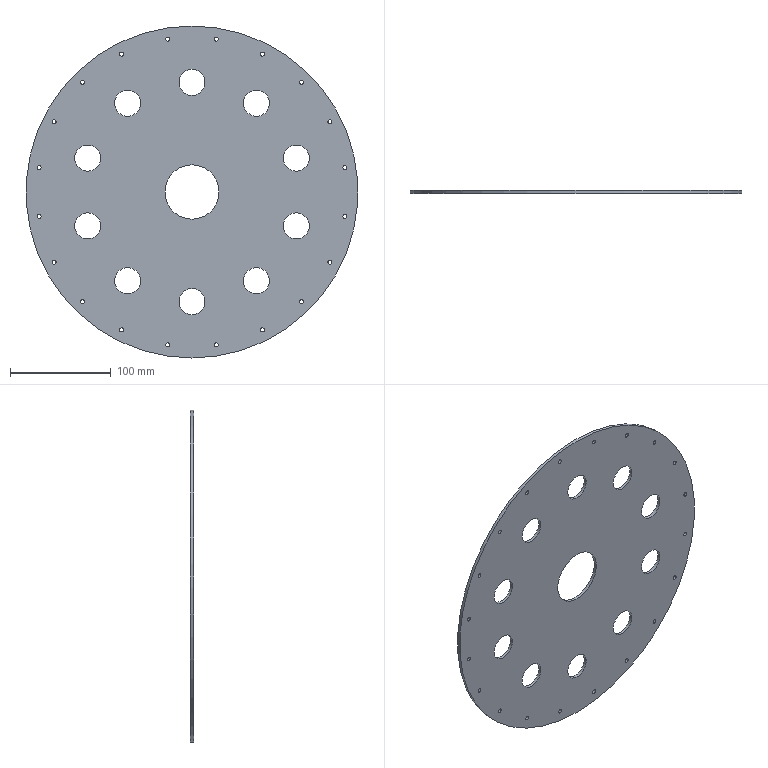Part | STEP file | JBJ-P-1012-05 | 1 solid | 34 faces | box 330 x 3 x 330 mm | volume 233037 mm3 | cylinder 32 | plane 2 | commonest cylinder face diameters 4 x20 26 x10 54 x1 330 x1
STEP:
#1=CARTESIAN_POINT('',(-24.,3.,-150.));
#2=VERTEX_POINT('',#1);
#3=CARTESIAN_POINT('',(-24.,3.,-152.));
#4=DIRECTION('',(0.,1.,0.));
#5=DIRECTION('',(0.,0.,1.));
#6=AXIS2_PLACEMENT_3D('',#3,#4,#5);
#7=CIRCLE('',#6,2.);
#8=EDGE_CURVE('',#2,#2,#7,.T.);
#9=ORIENTED_EDGE('',*,*,#8,.F.);
#10=EDGE_LOOP('',(#9));
#11=FACE_BOUND('',#10,.T.);
#12=CARTESIAN_POINT('',(24.,3.,-150.));
#13=VERTEX_POINT('',#12);
#14=CARTESIAN_POINT('',(24.,3.,-152.));
#15=DIRECTION('',(0.,1.,0.));
#16=DIRECTION('',(0.,0.,1.));
#17=AXIS2_PLACEMENT_3D('',#14,#15,#16);
#18=CIRCLE('',#17,2.);
#19=EDGE_CURVE('',#13,#13,#18,.T.);
#20=ORIENTED_EDGE('',*,*,#19,.F.);
#21=EDGE_LOOP('',(#20));
#22=FACE_BOUND('',#21,.T.);
#23=CARTESIAN_POINT('',(69.927,3.,-135.077));
#24=VERTEX_POINT('',#23);
#25=CARTESIAN_POINT('',(69.927,3.,-137.077));
#26=DIRECTION('',(0.,1.,0.));
#27=DIRECTION('',(0.,0.,1.));
#28=AXIS2_PLACEMENT_3D('',#25,#26,#27);
#29=CIRCLE('',#28,2.);
#30=EDGE_CURVE('',#24,#24,#29,.T.);
#31=ORIENTED_EDGE('',*,*,#30,.F.);
#32=EDGE_LOOP('',(#31));
#33=FACE_BOUND('',#32,.T.);
#34=CARTESIAN_POINT('',(108.76,3.,-106.864));
#35=VERTEX_POINT('',#34);
#36=CARTESIAN_POINT('',(108.76,3.,-108.864));
#37=DIRECTION('',(0.,1.,0.));
#38=DIRECTION('',(0.,0.,1.));
#39=AXIS2_PLACEMENT_3D('',#36,#37,#38);
#40=CIRCLE('',#39,2.);
#41=EDGE_CURVE('',#35,#35,#40,.T.);
#42=ORIENTED_EDGE('',*,*,#41,.F.);
#43=EDGE_LOOP('',(#42));
#44=FACE_BOUND('',#43,.T.);
#45=CARTESIAN_POINT('',(137.144,3.,-67.796));
#46=VERTEX_POINT('',#45);
#47=CARTESIAN_POINT('',(137.144,3.,-69.796));
#48=DIRECTION('',(0.,1.,0.));
#49=DIRECTION('',(0.,0.,1.));
#50=AXIS2_PLACEMENT_3D('',#47,#48,#49);
#51=CIRCLE('',#50,2.);
#52=EDGE_CURVE('',#46,#46,#51,.T.);
#53=ORIENTED_EDGE('',*,*,#52,.F.);
#54=EDGE_LOOP('',(#53));
#55=FACE_BOUND('',#54,.T.);
#56=CARTESIAN_POINT('',(151.977,3.,-22.145));
#57=VERTEX_POINT('',#56);
#58=CARTESIAN_POINT('',(151.977,3.,-24.145));
#59=DIRECTION('',(0.,1.,0.));
#60=DIRECTION('',(0.,0.,1.));
#61=AXIS2_PLACEMENT_3D('',#58,#59,#60);
#62=CIRCLE('',#61,2.);
#63=EDGE_CURVE('',#57,#57,#62,.T.);
#64=ORIENTED_EDGE('',*,*,#63,.F.);
#65=EDGE_LOOP('',(#64));
#66=FACE_BOUND('',#65,.T.);
#67=CARTESIAN_POINT('',(151.977,3.,26.145));
#68=VERTEX_POINT('',#67);
#69=CARTESIAN_POINT('',(151.977,3.,24.145));
#70=DIRECTION('',(0.,1.,0.));
#71=DIRECTION('',(0.,0.,1.));
#72=AXIS2_PLACEMENT_3D('',#69,#70,#71);
#73=CIRCLE('',#72,2.);
#74=EDGE_CURVE('',#68,#68,#73,.T.);
#75=ORIENTED_EDGE('',*,*,#74,.F.);
#76=EDGE_LOOP('',(#75));
#77=FACE_BOUND('',#76,.T.);
#78=CARTESIAN_POINT('',(137.144,3.,71.796));
#79=VERTEX_POINT('',#78);
#80=CARTESIAN_POINT('',(137.144,3.,69.796));
#81=DIRECTION('',(0.,1.,0.));
#82=DIRECTION('',(0.,0.,1.));
#83=AXIS2_PLACEMENT_3D('',#80,#81,#82);
#84=CIRCLE('',#83,2.);
#85=EDGE_CURVE('',#79,#79,#84,.T.);
#86=ORIENTED_EDGE('',*,*,#85,.F.);
#87=EDGE_LOOP('',(#86));
#88=FACE_BOUND('',#87,.T.);
#89=CARTESIAN_POINT('',(108.76,3.,110.864));
#90=VERTEX_POINT('',#89);
#91=CARTESIAN_POINT('',(108.76,3.,108.864));
#92=DIRECTION('',(0.,1.,0.));
#93=DIRECTION('',(0.,0.,1.));
#94=AXIS2_PLACEMENT_3D('',#91,#92,#93);
#95=CIRCLE('',#94,2.);
#96=EDGE_CURVE('',#90,#90,#95,.T.);
#97=ORIENTED_EDGE('',*,*,#96,.F.);
#98=EDGE_LOOP('',(#97));
#99=FACE_BOUND('',#98,.T.);
#100=CARTESIAN_POINT('',(69.927,3.,139.077));
#101=VERTEX_POINT('',#100);
#102=CARTESIAN_POINT('',(69.927,3.,137.077));
#103=DIRECTION('',(0.,1.,0.));
#104=DIRECTION('',(0.,0.,1.));
#105=AXIS2_PLACEMENT_3D('',#102,#103,#104);
#106=CIRCLE('',#105,2.);
#107=EDGE_CURVE('',#101,#101,#106,.T.);
#108=ORIENTED_EDGE('',*,*,#107,.F.);
#109=EDGE_LOOP('',(#108));
#110=FACE_BOUND('',#109,.T.);
#111=CARTESIAN_POINT('',(24.,3.,154.));
#112=VERTEX_POINT('',#111);
#113=CARTESIAN_POINT('',(24.,3.,152.));
#114=DIRECTION('',(0.,1.,0.));
#115=DIRECTION('',(0.,0.,1.));
#116=AXIS2_PLACEMENT_3D('',#113,#114,#115);
#117=CIRCLE('',#116,2.);
#118=EDGE_CURVE('',#112,#112,#117,.T.);
#119=ORIENTED_EDGE('',*,*,#118,.F.);
#120=EDGE_LOOP('',(#119));
#121=FACE_BOUND('',#120,.T.);
#122=CARTESIAN_POINT('',(-24.,3.,154.));
#123=VERTEX_POINT('',#122);
#124=CARTESIAN_POINT('',(-24.,3.,152.));
#125=DIRECTION('',(0.,1.,0.));
#126=DIRECTION('',(0.,0.,1.));
#127=AXIS2_PLACEMENT_3D('',#124,#125,#126);
#128=CIRCLE('',#127,2.);
#129=EDGE_CURVE('',#123,#123,#128,.T.);
#130=ORIENTED_EDGE('',*,*,#129,.F.);
#131=EDGE_LOOP('',(#130));
#132=FACE_BOUND('',#131,.T.);
#133=CARTESIAN_POINT('',(-69.927,3.,139.077));
#134=VERTEX_POINT('',#133);
#135=CARTESIAN_POINT('',(-69.927,3.,137.077));
#136=DIRECTION('',(0.,1.,0.));
#137=DIRECTION('',(0.,0.,1.));
#138=AXIS2_PLACEMENT_3D('',#135,#136,#137);
#139=CIRCLE('',#138,2.);
#140=EDGE_CURVE('',#134,#134,#139,.T.);
#141=ORIENTED_EDGE('',*,*,#140,.F.);
#142=EDGE_LOOP('',(#141));
#143=FACE_BOUND('',#142,.T.);
#144=CARTESIAN_POINT('',(-108.76,3.,110.864));
#145=VERTEX_POINT('',#144);
#146=CARTESIAN_POINT('',(-108.76,3.,108.864));
#147=DIRECTION('',(0.,1.,0.));
#148=DIRECTION('',(0.,0.,1.));
#149=AXIS2_PLACEMENT_3D('',#146,#147,#148);
#150=CIRCLE('',#149,2.);
#151=EDGE_CURVE('',#145,#145,#150,.T.);
#152=ORIENTED_EDGE('',*,*,#151,.F.);
#153=EDGE_LOOP('',(#152));
#154=FACE_BOUND('',#153,.T.);
#155=CARTESIAN_POINT('',(-137.144,3.,71.796));
#156=VERTEX_POINT('',#155);
#157=CARTESIAN_POINT('',(-137.144,3.,69.796));
#158=DIRECTION('',(0.,1.,0.));
#159=DIRECTION('',(0.,0.,1.));
#160=AXIS2_PLACEMENT_3D('',#157,#158,#159);
#161=CIRCLE('',#160,2.);
#162=EDGE_CURVE('',#156,#156,#161,.T.);
#163=ORIENTED_EDGE('',*,*,#162,.F.);
#164=EDGE_LOOP('',(#163));
#165=FACE_BOUND('',#164,.T.);
#166=CARTESIAN_POINT('',(-151.977,3.,26.145));
#167=VERTEX_POINT('',#166);
#168=CARTESIAN_POINT('',(-151.977,3.,24.145));
#169=DIRECTION('',(0.,1.,0.));
#170=DIRECTION('',(0.,0.,1.));
#171=AXIS2_PLACEMENT_3D('',#168,#169,#170);
#172=CIRCLE('',#171,2.);
#173=EDGE_CURVE('',#167,#167,#172,.T.);
#174=ORIENTED_EDGE('',*,*,#173,.F.);
#175=EDGE_LOOP('',(#174));
#176=FACE_BOUND('',#175,.T.);
#177=CARTESIAN_POINT('',(-151.977,3.,-22.145));
#178=VERTEX_POINT('',#177);
#179=CARTESIAN_POINT('',(-151.977,3.,-24.145));
#180=DIRECTION('',(0.,1.,0.));
#181=DIRECTION('',(0.,0.,1.));
#182=AXIS2_PLACEMENT_3D('',#179,#180,#181);
#183=CIRCLE('',#182,2.);
#184=EDGE_CURVE('',#178,#178,#183,.T.);
#185=ORIENTED_EDGE('',*,*,#184,.F.);
#186=EDGE_LOOP('',(#185));
#187=FACE_BOUND('',#186,.T.);
#188=CARTESIAN_POINT('',(-137.144,3.,-67.796));
#189=VERTEX_POINT('',#188);
#190=CARTESIAN_POINT('',(-137.144,3.,-69.796));
#191=DIRECTION('',(0.,1.,0.));
#192=DIRECTION('',(0.,0.,1.));
#193=AXIS2_PLACEMENT_3D('',#190,#191,#192);
#194=CIRCLE('',#193,2.);
#195=EDGE_CURVE('',#189,#189,#194,.T.);
#196=ORIENTED_EDGE('',*,*,#195,.F.);
#197=EDGE_LOOP('',(#196));
#198=FACE_BOUND('',#197,.T.);
#199=CARTESIAN_POINT('',(-108.76,3.,-106.864));
#200=VERTEX_POINT('',#199);
#201=CARTESIAN_POINT('',(-108.76,3.,-108.864));
#202=DIRECTION('',(0.,1.,0.));
#203=DIRECTION('',(0.,0.,1.));
#204=AXIS2_PLACEMENT_3D('',#201,#202,#203);
#205=CIRCLE('',#204,2.);
#206=EDGE_CURVE('',#200,#200,#205,.T.);
#207=ORIENTED_EDGE('',*,*,#206,.F.);
#208=EDGE_LOOP('',(#207));
#209=FACE_BOUND('',#208,.T.);
#210=CARTESIAN_POINT('',(-69.927,3.,-135.077));
#211=VERTEX_POINT('',#210);
#212=CARTESIAN_POINT('',(-69.927,3.,-137.077));
#213=DIRECTION('',(0.,1.,0.));
#214=DIRECTION('',(0.,0.,1.));
#215=AXIS2_PLACEMENT_3D('',#212,#213,#214);
#216=CIRCLE('',#215,2.);
#217=EDGE_CURVE('',#211,#211,#216,.T.);
#218=ORIENTED_EDGE('',*,*,#217,.F.);
#219=EDGE_LOOP('',(#218));
#220=FACE_BOUND('',#219,.T.);
#221=CARTESIAN_POINT('',(0.,3.,122.));
#222=VERTEX_POINT('',#221);
#223=CARTESIAN_POINT('',(0.,3.,109.));
#224=DIRECTION('',(0.,1.,0.));
#225=DIRECTION('',(0.,0.,1.));
#226=AXIS2_PLACEMENT_3D('',#223,#224,#225);
#227=CIRCLE('',#226,13.);
#228=EDGE_CURVE('',#222,#222,#227,.T.);
#229=ORIENTED_EDGE('',*,*,#228,.F.);
#230=EDGE_LOOP('',(#229));
#231=FACE_BOUND('',#230,.T.);
#232=CARTESIAN_POINT('',(103.665,3.,46.683));
#233=VERTEX_POINT('',#232);
#234=CARTESIAN_POINT('',(103.665,3.,33.683));
#235=DIRECTION('',(0.,1.,0.));
#236=DIRECTION('',(0.,0.,1.));
#237=AXIS2_PLACEMENT_3D('',#234,#235,#236);
#238=CIRCLE('',#237,13.);
#239=EDGE_CURVE('',#233,#233,#238,.T.);
#240=ORIENTED_EDGE('',*,*,#239,.F.);
#241=EDGE_LOOP('',(#240));
#242=FACE_BOUND('',#241,.T.);
#243=CARTESIAN_POINT('',(64.069,3.,-75.183));
#244=VERTEX_POINT('',#243);
#245=CARTESIAN_POINT('',(64.069,3.,-88.183));
#246=DIRECTION('',(0.,1.,0.));
#247=DIRECTION('',(0.,0.,1.));
#248=AXIS2_PLACEMENT_3D('',#245,#246,#247);
#249=CIRCLE('',#248,13.);
#250=EDGE_CURVE('',#244,#244,#249,.T.);
#251=ORIENTED_EDGE('',*,*,#250,.F.);
#252=EDGE_LOOP('',(#251));
#253=FACE_BOUND('',#252,.T.);
#254=CARTESIAN_POINT('',(-64.069,3.,-75.183));
#255=VERTEX_POINT('',#254);
#256=CARTESIAN_POINT('',(-64.069,3.,-88.183));
#257=DIRECTION('',(0.,1.,0.));
#258=DIRECTION('',(0.,0.,1.));
#259=AXIS2_PLACEMENT_3D('',#256,#257,#258);
#260=CIRCLE('',#259,13.);
#261=EDGE_CURVE('',#255,#255,#260,.T.);
#262=ORIENTED_EDGE('',*,*,#261,.F.);
#263=EDGE_LOOP('',(#262));
#264=FACE_BOUND('',#263,.T.);
#265=CARTESIAN_POINT('',(-103.665,3.,-20.683));
#266=VERTEX_POINT('',#265);
#267=CARTESIAN_POINT('',(-103.665,3.,-33.683));
#268=DIRECTION('',(0.,1.,0.));
#269=DIRECTION('',(0.,0.,1.));
#270=AXIS2_PLACEMENT_3D('',#267,#268,#269);
#271=CIRCLE('',#270,13.);
#272=EDGE_CURVE('',#266,#266,#271,.T.);
#273=ORIENTED_EDGE('',*,*,#272,.F.);
#274=EDGE_LOOP('',(#273));
#275=FACE_BOUND('',#274,.T.);
#276=CARTESIAN_POINT('',(0.,3.,165.));
#277=VERTEX_POINT('',#276);
#278=CARTESIAN_POINT('',(0.,3.,0.));
#279=DIRECTION('',(0.,1.,0.));
#280=DIRECTION('',(0.,0.,1.));
#281=AXIS2_PLACEMENT_3D('',#278,#279,#280);
#282=CIRCLE('',#281,165.);
#283=EDGE_CURVE('',#277,#277,#282,.T.);
#284=ORIENTED_EDGE('',*,*,#283,.T.);
#285=EDGE_LOOP('',(#284));
#286=FACE_OUTER_BOUND('',#285,.T.);
#287=CARTESIAN_POINT('',(0.,3.,27.));
#288=VERTEX_POINT('',#287);
#289=CARTESIAN_POINT('',(0.,3.,0.));
#290=DIRECTION('',(0.,1.,0.));
#291=DIRECTION('',(0.,0.,1.));
#292=AXIS2_PLACEMENT_3D('',#289,#290,#291);
#293=CIRCLE('',#292,27.);
#294=EDGE_CURVE('',#288,#288,#293,.T.);
#295=ORIENTED_EDGE('',*,*,#294,.F.);
#296=EDGE_LOOP('',(#295));
#297=FACE_BOUND('',#296,.T.);
#298=CARTESIAN_POINT('',(-103.665,3.,46.683));
#299=VERTEX_POINT('',#298);
#300=CARTESIAN_POINT('',(-103.665,3.,33.683));
#301=DIRECTION('',(0.,1.,0.));
#302=DIRECTION('',(0.,0.,1.));
#303=AXIS2_PLACEMENT_3D('',#300,#301,#302);
#304=CIRCLE('',#303,13.);
#305=EDGE_CURVE('',#299,#299,#304,.T.);
#306=ORIENTED_EDGE('',*,*,#305,.F.);
#307=EDGE_LOOP('',(#306));
#308=FACE_BOUND('',#307,.T.);
#309=CARTESIAN_POINT('',(0.,3.,-96.));
#310=VERTEX_POINT('',#309);
#311=CARTESIAN_POINT('',(0.,3.,-109.));
#312=DIRECTION('',(0.,1.,0.));
#313=DIRECTION('',(0.,0.,1.));
#314=AXIS2_PLACEMENT_3D('',#311,#312,#313);
#315=CIRCLE('',#314,13.);
#316=EDGE_CURVE('',#310,#310,#315,.T.);
#317=ORIENTED_EDGE('',*,*,#316,.F.);
#318=EDGE_LOOP('',(#317));
#319=FACE_BOUND('',#318,.T.);
#320=CARTESIAN_POINT('',(103.665,3.,-20.683));
#321=VERTEX_POINT('',#320);
#322=CARTESIAN_POINT('',(103.665,3.,-33.683));
#323=DIRECTION('',(0.,1.,0.));
#324=DIRECTION('',(0.,0.,1.));
#325=AXIS2_PLACEMENT_3D('',#322,#323,#324);
#326=CIRCLE('',#325,13.);
#327=EDGE_CURVE('',#321,#321,#326,.T.);
#328=ORIENTED_EDGE('',*,*,#327,.F.);
#329=EDGE_LOOP('',(#328));
#330=FACE_BOUND('',#329,.T.);
#331=CARTESIAN_POINT('',(64.069,3.,101.183));
#332=VERTEX_POINT('',#331);
#333=CARTESIAN_POINT('',(64.069,3.,88.183));
#334=DIRECTION('',(0.,1.,0.));
#335=DIRECTION('',(0.,0.,1.));
#336=AXIS2_PLACEMENT_3D('',#333,#334,#335);
#337=CIRCLE('',#336,13.);
#338=EDGE_CURVE('',#332,#332,#337,.T.);
#339=ORIENTED_EDGE('',*,*,#338,.F.);
#340=EDGE_LOOP('',(#339));
#341=FACE_BOUND('',#340,.T.);
#342=CARTESIAN_POINT('',(-64.069,3.,101.183));
#343=VERTEX_POINT('',#342);
#344=CARTESIAN_POINT('',(-64.069,3.,88.183));
#345=DIRECTION('',(0.,1.,0.));
#346=DIRECTION('',(0.,0.,1.));
#347=AXIS2_PLACEMENT_3D('',#344,#345,#346);
#348=CIRCLE('',#347,13.);
#349=EDGE_CURVE('',#343,#343,#348,.T.);
#350=ORIENTED_EDGE('',*,*,#349,.F.);
#351=EDGE_LOOP('',(#350));
#352=FACE_BOUND('',#351,.T.);
#353=CARTESIAN_POINT('',(0.,3.,0.));
#354=DIRECTION('',(0.,1.,0.));
#355=DIRECTION('',(0.,0.,1.));
#356=AXIS2_PLACEMENT_3D('',#353,#354,#355);
#357=PLANE('',#356);
#358=ADVANCED_FACE('',(#11,#22,#33,#44,#55,#66,#77,#88,#99,#110,#121,#132,#143,#154,#165,#176,#187,#198,#209,#220,#231,#242,#253,#264,#275,#286,#297,#308,#319,#330,#341,#352),#357,.T.);
#359=CARTESIAN_POINT('',(-24.,0.,-150.));
#360=VERTEX_POINT('',#359);
#361=CARTESIAN_POINT('',(-24.,0.,-152.));
#362=DIRECTION('',(0.,1.,0.));
#363=DIRECTION('',(0.,0.,1.));
#364=AXIS2_PLACEMENT_3D('',#361,#362,#363);
#365=CIRCLE('',#364,2.);
#366=EDGE_CURVE('',#360,#360,#365,.T.);
#367=ORIENTED_EDGE('',*,*,#366,.T.);
#368=EDGE_LOOP('',(#367));
#369=FACE_BOUND('',#368,.T.);
#370=CARTESIAN_POINT('',(24.,0.,-150.));
#371=VERTEX_POINT('',#370);
#372=CARTESIAN_POINT('',(24.,0.,-152.));
#373=DIRECTION('',(0.,1.,0.));
#374=DIRECTION('',(0.,0.,1.));
#375=AXIS2_PLACEMENT_3D('',#372,#373,#374);
#376=CIRCLE('',#375,2.);
#377=EDGE_CURVE('',#371,#371,#376,.T.);
#378=ORIENTED_EDGE('',*,*,#377,.T.);
#379=EDGE_LOOP('',(#378));
#380=FACE_BOUND('',#379,.T.);
#381=CARTESIAN_POINT('',(69.927,0.,-135.077));
#382=VERTEX_POINT('',#381);
#383=CARTESIAN_POINT('',(69.927,0.,-137.077));
#384=DIRECTION('',(0.,1.,0.));
#385=DIRECTION('',(0.,0.,1.));
#386=AXIS2_PLACEMENT_3D('',#383,#384,#385);
#387=CIRCLE('',#386,2.);
#388=EDGE_CURVE('',#382,#382,#387,.T.);
#389=ORIENTED_EDGE('',*,*,#388,.T.);
#390=EDGE_LOOP('',(#389));
#391=FACE_BOUND('',#390,.T.);
#392=CARTESIAN_POINT('',(108.76,0.,-106.864));
#393=VERTEX_POINT('',#392);
#394=CARTESIAN_POINT('',(108.76,0.,-108.864));
#395=DIRECTION('',(0.,1.,0.));
#396=DIRECTION('',(0.,0.,1.));
#397=AXIS2_PLACEMENT_3D('',#394,#395,#396);
#398=CIRCLE('',#397,2.);
#399=EDGE_CURVE('',#393,#393,#398,.T.);
#400=ORIENTED_EDGE('',*,*,#399,.T.);
#401=EDGE_LOOP('',(#400));
#402=FACE_BOUND('',#401,.T.);
#403=CARTESIAN_POINT('',(137.144,0.,-67.796));
#404=VERTEX_POINT('',#403);
#405=CARTESIAN_POINT('',(137.144,0.,-69.796));
#406=DIRECTION('',(0.,1.,0.));
#407=DIRECTION('',(0.,0.,1.));
#408=AXIS2_PLACEMENT_3D('',#405,#406,#407);
#409=CIRCLE('',#408,2.);
#410=EDGE_CURVE('',#404,#404,#409,.T.);
#411=ORIENTED_EDGE('',*,*,#410,.T.);
#412=EDGE_LOOP('',(#411));
#413=FACE_BOUND('',#412,.T.);
#414=CARTESIAN_POINT('',(151.977,0.,-22.145));
#415=VERTEX_POINT('',#414);
#416=CARTESIAN_POINT('',(151.977,0.,-24.145));
#417=DIRECTION('',(0.,1.,0.));
#418=DIRECTION('',(0.,0.,1.));
#419=AXIS2_PLACEMENT_3D('',#416,#417,#418);
#420=CIRCLE('',#419,2.);
#421=EDGE_CURVE('',#415,#415,#420,.T.);
#422=ORIENTED_EDGE('',*,*,#421,.T.);
#423=EDGE_LOOP('',(#422));
#424=FACE_BOUND('',#423,.T.);
#425=CARTESIAN_POINT('',(151.977,0.,26.145));
#426=VERTEX_POINT('',#425);
#427=CARTESIAN_POINT('',(151.977,0.,24.145));
#428=DIRECTION('',(0.,1.,0.));
#429=DIRECTION('',(0.,0.,1.));
#430=AXIS2_PLACEMENT_3D('',#427,#428,#429);
#431=CIRCLE('',#430,2.);
#432=EDGE_CURVE('',#426,#426,#431,.T.);
#433=ORIENTED_EDGE('',*,*,#432,.T.);
#434=EDGE_LOOP('',(#433));
#435=FACE_BOUND('',#434,.T.);
#436=CARTESIAN_POINT('',(137.144,0.,71.796));
#437=VERTEX_POINT('',#436);
#438=CARTESIAN_POINT('',(137.144,0.,69.796));
#439=DIRECTION('',(0.,1.,0.));
#440=DIRECTION('',(0.,0.,1.));
#441=AXIS2_PLACEMENT_3D('',#438,#439,#440);
#442=CIRCLE('',#441,2.);
#443=EDGE_CURVE('',#437,#437,#442,.T.);
#444=ORIENTED_EDGE('',*,*,#443,.T.);
#445=EDGE_LOOP('',(#444));
#446=FACE_BOUND('',#445,.T.);
#447=CARTESIAN_POINT('',(108.76,0.,110.864));
#448=VERTEX_POINT('',#447);
#449=CARTESIAN_POINT('',(108.76,0.,108.864));
#450=DIRECTION('',(0.,1.,0.));
#451=DIRECTION('',(0.,0.,1.));
#452=AXIS2_PLACEMENT_3D('',#449,#450,#451);
#453=CIRCLE('',#452,2.);
#454=EDGE_CURVE('',#448,#448,#453,.T.);
#455=ORIENTED_EDGE('',*,*,#454,.T.);
#456=EDGE_LOOP('',(#455));
#457=FACE_BOUND('',#456,.T.);
#458=CARTESIAN_POINT('',(69.927,0.,139.077));
#459=VERTEX_POINT('',#458);
#460=CARTESIAN_POINT('',(69.927,0.,137.077));
#461=DIRECTION('',(0.,1.,0.));
#462=DIRECTION('',(0.,0.,1.));
#463=AXIS2_PLACEMENT_3D('',#460,#461,#462);
#464=CIRCLE('',#463,2.);
#465=EDGE_CURVE('',#459,#459,#464,.T.);
#466=ORIENTED_EDGE('',*,*,#465,.T.);
#467=EDGE_LOOP('',(#466));
#468=FACE_BOUND('',#467,.T.);
#469=CARTESIAN_POINT('',(24.,0.,154.));
#470=VERTEX_POINT('',#469);
#471=CARTESIAN_POINT('',(24.,0.,152.));
#472=DIRECTION('',(0.,1.,0.));
#473=DIRECTION('',(0.,0.,1.));
#474=AXIS2_PLACEMENT_3D('',#471,#472,#473);
#475=CIRCLE('',#474,2.);
#476=EDGE_CURVE('',#470,#470,#475,.T.);
#477=ORIENTED_EDGE('',*,*,#476,.T.);
#478=EDGE_LOOP('',(#477));
#479=FACE_BOUND('',#478,.T.);
#480=CARTESIAN_POINT('',(-24.,0.,154.));
#481=VERTEX_POINT('',#480);
#482=CARTESIAN_POINT('',(-24.,0.,152.));
#483=DIRECTION('',(0.,1.,0.));
#484=DIRECTION('',(0.,0.,1.));
#485=AXIS2_PLACEMENT_3D('',#482,#483,#484);
#486=CIRCLE('',#485,2.);
#487=EDGE_CURVE('',#481,#481,#486,.T.);
#488=ORIENTED_EDGE('',*,*,#487,.T.);
#489=EDGE_LOOP('',(#488));
#490=FACE_BOUND('',#489,.T.);
#491=CARTESIAN_POINT('',(-69.927,0.,139.077));
#492=VERTEX_POINT('',#491);
#493=CARTESIAN_POINT('',(-69.927,0.,137.077));
#494=DIRECTION('',(0.,1.,0.));
#495=DIRECTION('',(0.,0.,1.));
#496=AXIS2_PLACEMENT_3D('',#493,#494,#495);
#497=CIRCLE('',#496,2.);
#498=EDGE_CURVE('',#492,#492,#497,.T.);
#499=ORIENTED_EDGE('',*,*,#498,.T.);
#500=EDGE_LOOP('',(#499));
#501=FACE_BOUND('',#500,.T.);
#502=CARTESIAN_POINT('',(-108.76,0.,110.864));
#503=VERTEX_POINT('',#502);
#504=CARTESIAN_POINT('',(-108.76,0.,108.864));
#505=DIRECTION('',(0.,1.,0.));
#506=DIRECTION('',(0.,0.,1.));
#507=AXIS2_PLACEMENT_3D('',#504,#505,#506);
#508=CIRCLE('',#507,2.);
#509=EDGE_CURVE('',#503,#503,#508,.T.);
#510=ORIENTED_EDGE('',*,*,#509,.T.);
#511=EDGE_LOOP('',(#510));
#512=FACE_BOUND('',#511,.T.);
#513=CARTESIAN_POINT('',(-137.144,0.,71.796));
#514=VERTEX_POINT('',#513);
#515=CARTESIAN_POINT('',(-137.144,0.,69.796));
#516=DIRECTION('',(0.,1.,0.));
#517=DIRECTION('',(0.,0.,1.));
#518=AXIS2_PLACEMENT_3D('',#515,#516,#517);
#519=CIRCLE('',#518,2.);
#520=EDGE_CURVE('',#514,#514,#519,.T.);
#521=ORIENTED_EDGE('',*,*,#520,.T.);
#522=EDGE_LOOP('',(#521));
#523=FACE_BOUND('',#522,.T.);
#524=CARTESIAN_POINT('',(-151.977,0.,26.145));
#525=VERTEX_POINT('',#524);
#526=CARTESIAN_POINT('',(-151.977,0.,24.145));
#527=DIRECTION('',(0.,1.,0.));
#528=DIRECTION('',(0.,0.,1.));
#529=AXIS2_PLACEMENT_3D('',#526,#527,#528);
#530=CIRCLE('',#529,2.);
#531=EDGE_CURVE('',#525,#525,#530,.T.);
#532=ORIENTED_EDGE('',*,*,#531,.T.);
#533=EDGE_LOOP('',(#532));
#534=FACE_BOUND('',#533,.T.);
#535=CARTESIAN_POINT('',(-151.977,0.,-22.145));
#536=VERTEX_POINT('',#535);
#537=CARTESIAN_POINT('',(-151.977,0.,-24.145));
#538=DIRECTION('',(0.,1.,0.));
#539=DIRECTION('',(0.,0.,1.));
#540=AXIS2_PLACEMENT_3D('',#537,#538,#539);
#541=CIRCLE('',#540,2.);
#542=EDGE_CURVE('',#536,#536,#541,.T.);
#543=ORIENTED_EDGE('',*,*,#542,.T.);
#544=EDGE_LOOP('',(#543));
#545=FACE_BOUND('',#544,.T.);
#546=CARTESIAN_POINT('',(-137.144,0.,-67.796));
#547=VERTEX_POINT('',#546);
#548=CARTESIAN_POINT('',(-137.144,0.,-69.796));
#549=DIRECTION('',(0.,1.,0.));
#550=DIRECTION('',(0.,0.,1.));
#551=AXIS2_PLACEMENT_3D('',#548,#549,#550);
#552=CIRCLE('',#551,2.);
#553=EDGE_CURVE('',#547,#547,#552,.T.);
#554=ORIENTED_EDGE('',*,*,#553,.T.);
#555=EDGE_LOOP('',(#554));
#556=FACE_BOUND('',#555,.T.);
#557=CARTESIAN_POINT('',(-108.76,0.,-106.864));
#558=VERTEX_POINT('',#557);
#559=CARTESIAN_POINT('',(-108.76,0.,-108.864));
#560=DIRECTION('',(0.,1.,0.));
#561=DIRECTION('',(0.,0.,1.));
#562=AXIS2_PLACEMENT_3D('',#559,#560,#561);
#563=CIRCLE('',#562,2.);
#564=EDGE_CURVE('',#558,#558,#563,.T.);
#565=ORIENTED_EDGE('',*,*,#564,.T.);
#566=EDGE_LOOP('',(#565));
#567=FACE_BOUND('',#566,.T.);
#568=CARTESIAN_POINT('',(-69.927,0.,-135.077));
#569=VERTEX_POINT('',#568);
#570=CARTESIAN_POINT('',(-69.927,0.,-137.077));
#571=DIRECTION('',(0.,1.,0.));
#572=DIRECTION('',(0.,0.,1.));
#573=AXIS2_PLACEMENT_3D('',#570,#571,#572);
#574=CIRCLE('',#573,2.);
#575=EDGE_CURVE('',#569,#569,#574,.T.);
#576=ORIENTED_EDGE('',*,*,#575,.T.);
#577=EDGE_LOOP('',(#576));
#578=FACE_BOUND('',#577,.T.);
#579=CARTESIAN_POINT('',(0.,0.,165.));
#580=VERTEX_POINT('',#579);
#581=CARTESIAN_POINT('',(0.,0.,0.));
#582=DIRECTION('',(0.,1.,0.));
#583=DIRECTION('',(0.,0.,1.));
#584=AXIS2_PLACEMENT_3D('',#581,#582,#583);
#585=CIRCLE('',#584,165.);
#586=EDGE_CURVE('',#580,#580,#585,.T.);
#587=ORIENTED_EDGE('',*,*,#586,.F.);
#588=EDGE_LOOP('',(#587));
#589=FACE_OUTER_BOUND('',#588,.T.);
#590=CARTESIAN_POINT('',(0.,0.,27.));
#591=VERTEX_POINT('',#590);
#592=CARTESIAN_POINT('',(0.,0.,0.));
#593=DIRECTION('',(0.,1.,0.));
#594=DIRECTION('',(0.,0.,1.));
#595=AXIS2_PLACEMENT_3D('',#592,#593,#594);
#596=CIRCLE('',#595,27.);
#597=EDGE_CURVE('',#591,#591,#596,.T.);
#598=ORIENTED_EDGE('',*,*,#597,.T.);
#599=EDGE_LOOP('',(#598));
#600=FACE_BOUND('',#599,.T.);
#601=CARTESIAN_POINT('',(-103.665,0.,-20.683));
#602=VERTEX_POINT('',#601);
#603=CARTESIAN_POINT('',(-103.665,0.,-33.683));
#604=DIRECTION('',(0.,1.,0.));
#605=DIRECTION('',(0.,0.,1.));
#606=AXIS2_PLACEMENT_3D('',#603,#604,#605);
#607=CIRCLE('',#606,13.);
#608=EDGE_CURVE('',#602,#602,#607,.T.);
#609=ORIENTED_EDGE('',*,*,#608,.T.);
#610=EDGE_LOOP('',(#609));
#611=FACE_BOUND('',#610,.T.);
#612=CARTESIAN_POINT('',(-103.665,0.,46.683));
#613=VERTEX_POINT('',#612);
#614=CARTESIAN_POINT('',(-103.665,0.,33.683));
#615=DIRECTION('',(0.,1.,0.));
#616=DIRECTION('',(0.,0.,1.));
#617=AXIS2_PLACEMENT_3D('',#614,#615,#616);
#618=CIRCLE('',#617,13.);
#619=EDGE_CURVE('',#613,#613,#618,.T.);
#620=ORIENTED_EDGE('',*,*,#619,.T.);
#621=EDGE_LOOP('',(#620));
#622=FACE_BOUND('',#621,.T.);
#623=CARTESIAN_POINT('',(-64.069,0.,-75.183));
#624=VERTEX_POINT('',#623);
#625=CARTESIAN_POINT('',(-64.069,0.,-88.183));
#626=DIRECTION('',(0.,1.,0.));
#627=DIRECTION('',(0.,0.,1.));
#628=AXIS2_PLACEMENT_3D('',#625,#626,#627);
#629=CIRCLE('',#628,13.);
#630=EDGE_CURVE('',#624,#624,#629,.T.);
#631=ORIENTED_EDGE('',*,*,#630,.T.);
#632=EDGE_LOOP('',(#631));
#633=FACE_BOUND('',#632,.T.);
#634=CARTESIAN_POINT('',(0.,0.,-96.));
#635=VERTEX_POINT('',#634);
#636=CARTESIAN_POINT('',(0.,0.,-109.));
#637=DIRECTION('',(0.,1.,0.));
#638=DIRECTION('',(0.,0.,1.));
#639=AXIS2_PLACEMENT_3D('',#636,#637,#638);
#640=CIRCLE('',#639,13.);
#641=EDGE_CURVE('',#635,#635,#640,.T.);
#642=ORIENTED_EDGE('',*,*,#641,.T.);
#643=EDGE_LOOP('',(#642));
#644=FACE_BOUND('',#643,.T.);
#645=CARTESIAN_POINT('',(64.069,0.,-75.183));
#646=VERTEX_POINT('',#645);
#647=CARTESIAN_POINT('',(64.069,0.,-88.183));
#648=DIRECTION('',(0.,1.,0.));
#649=DIRECTION('',(0.,0.,1.));
#650=AXIS2_PLACEMENT_3D('',#647,#648,#649);
#651=CIRCLE('',#650,13.);
#652=EDGE_CURVE('',#646,#646,#651,.T.);
#653=ORIENTED_EDGE('',*,*,#652,.T.);
#654=EDGE_LOOP('',(#653));
#655=FACE_BOUND('',#654,.T.);
#656=CARTESIAN_POINT('',(103.665,0.,-20.683));
#657=VERTEX_POINT('',#656);
#658=CARTESIAN_POINT('',(103.665,0.,-33.683));
#659=DIRECTION('',(0.,1.,0.));
#660=DIRECTION('',(0.,0.,1.));
#661=AXIS2_PLACEMENT_3D('',#658,#659,#660);
#662=CIRCLE('',#661,13.);
#663=EDGE_CURVE('',#657,#657,#662,.T.);
#664=ORIENTED_EDGE('',*,*,#663,.T.);
#665=EDGE_LOOP('',(#664));
#666=FACE_BOUND('',#665,.T.);
#667=CARTESIAN_POINT('',(103.665,0.,46.683));
#668=VERTEX_POINT('',#667);
#669=CARTESIAN_POINT('',(103.665,0.,33.683));
#670=DIRECTION('',(0.,1.,0.));
#671=DIRECTION('',(0.,0.,1.));
#672=AXIS2_PLACEMENT_3D('',#669,#670,#671);
#673=CIRCLE('',#672,13.);
#674=EDGE_CURVE('',#668,#668,#673,.T.);
#675=ORIENTED_EDGE('',*,*,#674,.T.);
#676=EDGE_LOOP('',(#675));
#677=FACE_BOUND('',#676,.T.);
#678=CARTESIAN_POINT('',(64.069,0.,101.183));
#679=VERTEX_POINT('',#678);
#680=CARTESIAN_POINT('',(64.069,0.,88.183));
#681=DIRECTION('',(0.,1.,0.));
#682=DIRECTION('',(0.,0.,1.));
#683=AXIS2_PLACEMENT_3D('',#680,#681,#682);
#684=CIRCLE('',#683,13.);
#685=EDGE_CURVE('',#679,#679,#684,.T.);
#686=ORIENTED_EDGE('',*,*,#685,.T.);
#687=EDGE_LOOP('',(#686));
#688=FACE_BOUND('',#687,.T.);
#689=CARTESIAN_POINT('',(0.,0.,122.));
#690=VERTEX_POINT('',#689);
#691=CARTESIAN_POINT('',(0.,0.,109.));
#692=DIRECTION('',(0.,1.,0.));
#693=DIRECTION('',(0.,0.,1.));
#694=AXIS2_PLACEMENT_3D('',#691,#692,#693);
#695=CIRCLE('',#694,13.);
#696=EDGE_CURVE('',#690,#690,#695,.T.);
#697=ORIENTED_EDGE('',*,*,#696,.T.);
#698=EDGE_LOOP('',(#697));
#699=FACE_BOUND('',#698,.T.);
#700=CARTESIAN_POINT('',(-64.069,0.,101.183));
#701=VERTEX_POINT('',#700);
#702=CARTESIAN_POINT('',(-64.069,0.,88.183));
#703=DIRECTION('',(0.,1.,0.));
#704=DIRECTION('',(0.,0.,1.));
#705=AXIS2_PLACEMENT_3D('',#702,#703,#704);
#706=CIRCLE('',#705,13.);
#707=EDGE_CURVE('',#701,#701,#706,.T.);
#708=ORIENTED_EDGE('',*,*,#707,.T.);
#709=EDGE_LOOP('',(#708));
#710=FACE_BOUND('',#709,.T.);
#711=CARTESIAN_POINT('',(0.,0.,0.));
#712=DIRECTION('',(0.,1.,0.));
#713=DIRECTION('',(0.,0.,1.));
#714=AXIS2_PLACEMENT_3D('',#711,#712,#713);
#715=PLANE('',#714);
#716=ADVANCED_FACE('',(#369,#380,#391,#402,#413,#424,#435,#446,#457,#468,#479,#490,#501,#512,#523,#534,#545,#556,#567,#578,#589,#600,#611,#622,#633,#644,#655,#666,#677,#688,#699,#710),#715,.F.);
#717=ORIENTED_EDGE('',*,*,#283,.F.);
#718=EDGE_LOOP('',(#717));
#719=FACE_OUTER_BOUND('',#718,.T.);
#720=ORIENTED_EDGE('',*,*,#586,.T.);
#721=EDGE_LOOP('',(#720));
#722=FACE_OUTER_BOUND('',#721,.T.);
#723=CARTESIAN_POINT('',(0.,3.,0.));
#724=DIRECTION('',(0.,-1.,0.));
#725=DIRECTION('',(0.,0.,-1.));
#726=AXIS2_PLACEMENT_3D('',#723,#724,#725);
#727=CYLINDRICAL_SURFACE('',#726,165.);
#728=ADVANCED_FACE('',(#719,#722),#727,.T.);
#729=ORIENTED_EDGE('',*,*,#294,.T.);
#730=EDGE_LOOP('',(#729));
#731=FACE_OUTER_BOUND('',#730,.T.);
#732=ORIENTED_EDGE('',*,*,#597,.F.);
#733=EDGE_LOOP('',(#732));
#734=FACE_OUTER_BOUND('',#733,.T.);
#735=CARTESIAN_POINT('',(0.,3.,0.));
#736=DIRECTION('',(0.,-1.,0.));
#737=DIRECTION('',(0.,0.,-1.));
#738=AXIS2_PLACEMENT_3D('',#735,#736,#737);
#739=CYLINDRICAL_SURFACE('',#738,27.);
#740=ADVANCED_FACE('',(#731,#734),#739,.F.);
#741=ORIENTED_EDGE('',*,*,#272,.T.);
#742=EDGE_LOOP('',(#741));
#743=FACE_OUTER_BOUND('',#742,.T.);
#744=ORIENTED_EDGE('',*,*,#608,.F.);
#745=EDGE_LOOP('',(#744));
#746=FACE_OUTER_BOUND('',#745,.T.);
#747=CARTESIAN_POINT('',(-103.665,3.,-33.683));
#748=DIRECTION('',(0.,-1.,0.));
#749=DIRECTION('',(0.,0.,-1.));
#750=AXIS2_PLACEMENT_3D('',#747,#748,#749);
#751=CYLINDRICAL_SURFACE('',#750,13.);
#752=ADVANCED_FACE('',(#743,#746),#751,.F.);
#753=ORIENTED_EDGE('',*,*,#305,.T.);
#754=EDGE_LOOP('',(#753));
#755=FACE_OUTER_BOUND('',#754,.T.);
#756=ORIENTED_EDGE('',*,*,#619,.F.);
#757=EDGE_LOOP('',(#756));
#758=FACE_OUTER_BOUND('',#757,.T.);
#759=CARTESIAN_POINT('',(-103.665,3.,33.683));
#760=DIRECTION('',(0.,-1.,0.));
#761=DIRECTION('',(0.,0.,-1.));
#762=AXIS2_PLACEMENT_3D('',#759,#760,#761);
#763=CYLINDRICAL_SURFACE('',#762,13.);
#764=ADVANCED_FACE('',(#755,#758),#763,.F.);
#765=ORIENTED_EDGE('',*,*,#261,.T.);
#766=EDGE_LOOP('',(#765));
#767=FACE_OUTER_BOUND('',#766,.T.);
#768=ORIENTED_EDGE('',*,*,#630,.F.);
#769=EDGE_LOOP('',(#768));
#770=FACE_OUTER_BOUND('',#769,.T.);
#771=CARTESIAN_POINT('',(-64.069,3.,-88.183));
#772=DIRECTION('',(0.,-1.,0.));
#773=DIRECTION('',(0.,0.,-1.));
#774=AXIS2_PLACEMENT_3D('',#771,#772,#773);
#775=CYLINDRICAL_SURFACE('',#774,13.);
#776=ADVANCED_FACE('',(#767,#770),#775,.F.);
#777=ORIENTED_EDGE('',*,*,#316,.T.);
#778=EDGE_LOOP('',(#777));
#779=FACE_OUTER_BOUND('',#778,.T.);
#780=ORIENTED_EDGE('',*,*,#641,.F.);
#781=EDGE_LOOP('',(#780));
#782=FACE_OUTER_BOUND('',#781,.T.);
#783=CARTESIAN_POINT('',(0.,3.,-109.));
#784=DIRECTION('',(0.,-1.,0.));
#785=DIRECTION('',(0.,0.,-1.));
#786=AXIS2_PLACEMENT_3D('',#783,#784,#785);
#787=CYLINDRICAL_SURFACE('',#786,13.);
#788=ADVANCED_FACE('',(#779,#782),#787,.F.);
#789=ORIENTED_EDGE('',*,*,#250,.T.);
#790=EDGE_LOOP('',(#789));
#791=FACE_OUTER_BOUND('',#790,.T.);
#792=ORIENTED_EDGE('',*,*,#652,.F.);
#793=EDGE_LOOP('',(#792));
#794=FACE_OUTER_BOUND('',#793,.T.);
#795=CARTESIAN_POINT('',(64.069,3.,-88.183));
#796=DIRECTION('',(0.,-1.,0.));
#797=DIRECTION('',(0.,0.,-1.));
#798=AXIS2_PLACEMENT_3D('',#795,#796,#797);
#799=CYLINDRICAL_SURFACE('',#798,13.);
#800=ADVANCED_FACE('',(#791,#794),#799,.F.);
#801=ORIENTED_EDGE('',*,*,#327,.T.);
#802=EDGE_LOOP('',(#801));
#803=FACE_OUTER_BOUND('',#802,.T.);
#804=ORIENTED_EDGE('',*,*,#663,.F.);
#805=EDGE_LOOP('',(#804));
#806=FACE_OUTER_BOUND('',#805,.T.);
#807=CARTESIAN_POINT('',(103.665,3.,-33.683));
#808=DIRECTION('',(0.,-1.,0.));
#809=DIRECTION('',(0.,0.,-1.));
#810=AXIS2_PLACEMENT_3D('',#807,#808,#809);
#811=CYLINDRICAL_SURFACE('',#810,13.);
#812=ADVANCED_FACE('',(#803,#806),#811,.F.);
#813=ORIENTED_EDGE('',*,*,#239,.T.);
#814=EDGE_LOOP('',(#813));
#815=FACE_OUTER_BOUND('',#814,.T.);
#816=ORIENTED_EDGE('',*,*,#674,.F.);
#817=EDGE_LOOP('',(#816));
#818=FACE_OUTER_BOUND('',#817,.T.);
#819=CARTESIAN_POINT('',(103.665,3.,33.683));
#820=DIRECTION('',(0.,-1.,0.));
#821=DIRECTION('',(0.,0.,-1.));
#822=AXIS2_PLACEMENT_3D('',#819,#820,#821);
#823=CYLINDRICAL_SURFACE('',#822,13.);
#824=ADVANCED_FACE('',(#815,#818),#823,.F.);
#825=ORIENTED_EDGE('',*,*,#338,.T.);
#826=EDGE_LOOP('',(#825));
#827=FACE_OUTER_BOUND('',#826,.T.);
#828=ORIENTED_EDGE('',*,*,#685,.F.);
#829=EDGE_LOOP('',(#828));
#830=FACE_OUTER_BOUND('',#829,.T.);
#831=CARTESIAN_POINT('',(64.069,3.,88.183));
#832=DIRECTION('',(0.,-1.,0.));
#833=DIRECTION('',(0.,0.,-1.));
#834=AXIS2_PLACEMENT_3D('',#831,#832,#833);
#835=CYLINDRICAL_SURFACE('',#834,13.);
#836=ADVANCED_FACE('',(#827,#830),#835,.F.);
#837=ORIENTED_EDGE('',*,*,#228,.T.);
#838=EDGE_LOOP('',(#837));
#839=FACE_OUTER_BOUND('',#838,.T.);
#840=ORIENTED_EDGE('',*,*,#696,.F.);
#841=EDGE_LOOP('',(#840));
#842=FACE_OUTER_BOUND('',#841,.T.);
#843=CARTESIAN_POINT('',(0.,3.,109.));
#844=DIRECTION('',(0.,-1.,0.));
#845=DIRECTION('',(0.,0.,-1.));
#846=AXIS2_PLACEMENT_3D('',#843,#844,#845);
#847=CYLINDRICAL_SURFACE('',#846,13.);
#848=ADVANCED_FACE('',(#839,#842),#847,.F.);
#849=ORIENTED_EDGE('',*,*,#349,.T.);
#850=EDGE_LOOP('',(#849));
#851=FACE_OUTER_BOUND('',#850,.T.);
#852=ORIENTED_EDGE('',*,*,#707,.F.);
#853=EDGE_LOOP('',(#852));
#854=FACE_OUTER_BOUND('',#853,.T.);
#855=CARTESIAN_POINT('',(-64.069,3.,88.183));
#856=DIRECTION('',(0.,-1.,0.));
#857=DIRECTION('',(0.,0.,-1.));
#858=AXIS2_PLACEMENT_3D('',#855,#856,#857);
#859=CYLINDRICAL_SURFACE('',#858,13.);
#860=ADVANCED_FACE('',(#851,#854),#859,.F.);
#861=ORIENTED_EDGE('',*,*,#217,.T.);
#862=EDGE_LOOP('',(#861));
#863=FACE_OUTER_BOUND('',#862,.T.);
#864=ORIENTED_EDGE('',*,*,#575,.F.);
#865=EDGE_LOOP('',(#864));
#866=FACE_OUTER_BOUND('',#865,.T.);
#867=CARTESIAN_POINT('',(-69.927,3.,-137.077));
#868=DIRECTION('',(0.,1.,0.));
#869=DIRECTION('',(0.,0.,1.));
#870=AXIS2_PLACEMENT_3D('',#867,#868,#869);
#871=CYLINDRICAL_SURFACE('',#870,2.);
#872=ADVANCED_FACE('',(#863,#866),#871,.F.);
#873=ORIENTED_EDGE('',*,*,#206,.T.);
#874=EDGE_LOOP('',(#873));
#875=FACE_OUTER_BOUND('',#874,.T.);
#876=ORIENTED_EDGE('',*,*,#564,.F.);
#877=EDGE_LOOP('',(#876));
#878=FACE_OUTER_BOUND('',#877,.T.);
#879=CARTESIAN_POINT('',(-108.76,3.,-108.864));
#880=DIRECTION('',(0.,1.,0.));
#881=DIRECTION('',(0.,0.,1.));
#882=AXIS2_PLACEMENT_3D('',#879,#880,#881);
#883=CYLINDRICAL_SURFACE('',#882,2.);
#884=ADVANCED_FACE('',(#875,#878),#883,.F.);
#885=ORIENTED_EDGE('',*,*,#195,.T.);
#886=EDGE_LOOP('',(#885));
#887=FACE_OUTER_BOUND('',#886,.T.);
#888=ORIENTED_EDGE('',*,*,#553,.F.);
#889=EDGE_LOOP('',(#888));
#890=FACE_OUTER_BOUND('',#889,.T.);
#891=CARTESIAN_POINT('',(-137.144,3.,-69.796));
#892=DIRECTION('',(0.,1.,0.));
#893=DIRECTION('',(0.,0.,1.));
#894=AXIS2_PLACEMENT_3D('',#891,#892,#893);
#895=CYLINDRICAL_SURFACE('',#894,2.);
#896=ADVANCED_FACE('',(#887,#890),#895,.F.);
#897=ORIENTED_EDGE('',*,*,#184,.T.);
#898=EDGE_LOOP('',(#897));
#899=FACE_OUTER_BOUND('',#898,.T.);
#900=ORIENTED_EDGE('',*,*,#542,.F.);
#901=EDGE_LOOP('',(#900));
#902=FACE_OUTER_BOUND('',#901,.T.);
#903=CARTESIAN_POINT('',(-151.977,3.,-24.145));
#904=DIRECTION('',(0.,1.,0.));
#905=DIRECTION('',(0.,0.,1.));
#906=AXIS2_PLACEMENT_3D('',#903,#904,#905);
#907=CYLINDRICAL_SURFACE('',#906,2.);
#908=ADVANCED_FACE('',(#899,#902),#907,.F.);
#909=ORIENTED_EDGE('',*,*,#173,.T.);
#910=EDGE_LOOP('',(#909));
#911=FACE_OUTER_BOUND('',#910,.T.);
#912=ORIENTED_EDGE('',*,*,#531,.F.);
#913=EDGE_LOOP('',(#912));
#914=FACE_OUTER_BOUND('',#913,.T.);
#915=CARTESIAN_POINT('',(-151.977,3.,24.145));
#916=DIRECTION('',(0.,1.,0.));
#917=DIRECTION('',(0.,0.,1.));
#918=AXIS2_PLACEMENT_3D('',#915,#916,#917);
#919=CYLINDRICAL_SURFACE('',#918,2.);
#920=ADVANCED_FACE('',(#911,#914),#919,.F.);
#921=ORIENTED_EDGE('',*,*,#162,.T.);
#922=EDGE_LOOP('',(#921));
#923=FACE_OUTER_BOUND('',#922,.T.);
#924=ORIENTED_EDGE('',*,*,#520,.F.);
#925=EDGE_LOOP('',(#924));
#926=FACE_OUTER_BOUND('',#925,.T.);
#927=CARTESIAN_POINT('',(-137.144,3.,69.796));
#928=DIRECTION('',(0.,1.,0.));
#929=DIRECTION('',(0.,0.,1.));
#930=AXIS2_PLACEMENT_3D('',#927,#928,#929);
#931=CYLINDRICAL_SURFACE('',#930,2.);
#932=ADVANCED_FACE('',(#923,#926),#931,.F.);
#933=ORIENTED_EDGE('',*,*,#151,.T.);
#934=EDGE_LOOP('',(#933));
#935=FACE_OUTER_BOUND('',#934,.T.);
#936=ORIENTED_EDGE('',*,*,#509,.F.);
#937=EDGE_LOOP('',(#936));
#938=FACE_OUTER_BOUND('',#937,.T.);
#939=CARTESIAN_POINT('',(-108.76,3.,108.864));
#940=DIRECTION('',(0.,1.,0.));
#941=DIRECTION('',(0.,0.,1.));
#942=AXIS2_PLACEMENT_3D('',#939,#940,#941);
#943=CYLINDRICAL_SURFACE('',#942,2.);
#944=ADVANCED_FACE('',(#935,#938),#943,.F.);
#945=ORIENTED_EDGE('',*,*,#140,.T.);
#946=EDGE_LOOP('',(#945));
#947=FACE_OUTER_BOUND('',#946,.T.);
#948=ORIENTED_EDGE('',*,*,#498,.F.);
#949=EDGE_LOOP('',(#948));
#950=FACE_OUTER_BOUND('',#949,.T.);
#951=CARTESIAN_POINT('',(-69.927,3.,137.077));
#952=DIRECTION('',(0.,1.,0.));
#953=DIRECTION('',(0.,0.,1.));
#954=AXIS2_PLACEMENT_3D('',#951,#952,#953);
#955=CYLINDRICAL_SURFACE('',#954,2.);
#956=ADVANCED_FACE('',(#947,#950),#955,.F.);
#957=ORIENTED_EDGE('',*,*,#129,.T.);
#958=EDGE_LOOP('',(#957));
#959=FACE_OUTER_BOUND('',#958,.T.);
#960=ORIENTED_EDGE('',*,*,#487,.F.);
#961=EDGE_LOOP('',(#960));
#962=FACE_OUTER_BOUND('',#961,.T.);
#963=CARTESIAN_POINT('',(-24.,3.,152.));
#964=DIRECTION('',(0.,1.,0.));
#965=DIRECTION('',(0.,0.,1.));
#966=AXIS2_PLACEMENT_3D('',#963,#964,#965);
#967=CYLINDRICAL_SURFACE('',#966,2.);
#968=ADVANCED_FACE('',(#959,#962),#967,.F.);
#969=ORIENTED_EDGE('',*,*,#118,.T.);
#970=EDGE_LOOP('',(#969));
#971=FACE_OUTER_BOUND('',#970,.T.);
#972=ORIENTED_EDGE('',*,*,#476,.F.);
#973=EDGE_LOOP('',(#972));
#974=FACE_OUTER_BOUND('',#973,.T.);
#975=CARTESIAN_POINT('',(24.,3.,152.));
#976=DIRECTION('',(0.,1.,0.));
#977=DIRECTION('',(0.,0.,1.));
#978=AXIS2_PLACEMENT_3D('',#975,#976,#977);
#979=CYLINDRICAL_SURFACE('',#978,2.);
#980=ADVANCED_FACE('',(#971,#974),#979,.F.);
#981=ORIENTED_EDGE('',*,*,#107,.T.);
#982=EDGE_LOOP('',(#981));
#983=FACE_OUTER_BOUND('',#982,.T.);
#984=ORIENTED_EDGE('',*,*,#465,.F.);
#985=EDGE_LOOP('',(#984));
#986=FACE_OUTER_BOUND('',#985,.T.);
#987=CARTESIAN_POINT('',(69.927,3.,137.077));
#988=DIRECTION('',(0.,1.,0.));
#989=DIRECTION('',(0.,0.,1.));
#990=AXIS2_PLACEMENT_3D('',#987,#988,#989);
#991=CYLINDRICAL_SURFACE('',#990,2.);
#992=ADVANCED_FACE('',(#983,#986),#991,.F.);
#993=ORIENTED_EDGE('',*,*,#96,.T.);
#994=EDGE_LOOP('',(#993));
#995=FACE_OUTER_BOUND('',#994,.T.);
#996=ORIENTED_EDGE('',*,*,#454,.F.);
#997=EDGE_LOOP('',(#996));
#998=FACE_OUTER_BOUND('',#997,.T.);
#999=CARTESIAN_POINT('',(108.76,3.,108.864));
#1000=DIRECTION('',(0.,1.,0.));
#1001=DIRECTION('',(0.,0.,1.));
#1002=AXIS2_PLACEMENT_3D('',#999,#1000,#1001);
#1003=CYLINDRICAL_SURFACE('',#1002,2.);
#1004=ADVANCED_FACE('',(#995,#998),#1003,.F.);
#1005=ORIENTED_EDGE('',*,*,#85,.T.);
#1006=EDGE_LOOP('',(#1005));
#1007=FACE_OUTER_BOUND('',#1006,.T.);
#1008=ORIENTED_EDGE('',*,*,#443,.F.);
#1009=EDGE_LOOP('',(#1008));
#1010=FACE_OUTER_BOUND('',#1009,.T.);
#1011=CARTESIAN_POINT('',(137.144,3.,69.796));
#1012=DIRECTION('',(0.,1.,0.));
#1013=DIRECTION('',(0.,0.,1.));
#1014=AXIS2_PLACEMENT_3D('',#1011,#1012,#1013);
#1015=CYLINDRICAL_SURFACE('',#1014,2.);
#1016=ADVANCED_FACE('',(#1007,#1010),#1015,.F.);
#1017=ORIENTED_EDGE('',*,*,#74,.T.);
#1018=EDGE_LOOP('',(#1017));
#1019=FACE_OUTER_BOUND('',#1018,.T.);
#1020=ORIENTED_EDGE('',*,*,#432,.F.);
#1021=EDGE_LOOP('',(#1020));
#1022=FACE_OUTER_BOUND('',#1021,.T.);
#1023=CARTESIAN_POINT('',(151.977,3.,24.145));
#1024=DIRECTION('',(0.,1.,0.));
#1025=DIRECTION('',(0.,0.,1.));
#1026=AXIS2_PLACEMENT_3D('',#1023,#1024,#1025);
#1027=CYLINDRICAL_SURFACE('',#1026,2.);
#1028=ADVANCED_FACE('',(#1019,#1022),#1027,.F.);
#1029=ORIENTED_EDGE('',*,*,#63,.T.);
#1030=EDGE_LOOP('',(#1029));
#1031=FACE_OUTER_BOUND('',#1030,.T.);
#1032=ORIENTED_EDGE('',*,*,#421,.F.);
#1033=EDGE_LOOP('',(#1032));
#1034=FACE_OUTER_BOUND('',#1033,.T.);
#1035=CARTESIAN_POINT('',(151.977,3.,-24.145));
#1036=DIRECTION('',(0.,1.,0.));
#1037=DIRECTION('',(0.,0.,1.));
#1038=AXIS2_PLACEMENT_3D('',#1035,#1036,#1037);
#1039=CYLINDRICAL_SURFACE('',#1038,2.);
#1040=ADVANCED_FACE('',(#1031,#1034),#1039,.F.);
#1041=ORIENTED_EDGE('',*,*,#52,.T.);
#1042=EDGE_LOOP('',(#1041));
#1043=FACE_OUTER_BOUND('',#1042,.T.);
#1044=ORIENTED_EDGE('',*,*,#410,.F.);
#1045=EDGE_LOOP('',(#1044));
#1046=FACE_OUTER_BOUND('',#1045,.T.);
#1047=CARTESIAN_POINT('',(137.144,3.,-69.796));
#1048=DIRECTION('',(0.,1.,0.));
#1049=DIRECTION('',(0.,0.,1.));
#1050=AXIS2_PLACEMENT_3D('',#1047,#1048,#1049);
#1051=CYLINDRICAL_SURFACE('',#1050,2.);
#1052=ADVANCED_FACE('',(#1043,#1046),#1051,.F.);
#1053=ORIENTED_EDGE('',*,*,#41,.T.);
#1054=EDGE_LOOP('',(#1053));
#1055=FACE_OUTER_BOUND('',#1054,.T.);
#1056=ORIENTED_EDGE('',*,*,#399,.F.);
#1057=EDGE_LOOP('',(#1056));
#1058=FACE_OUTER_BOUND('',#1057,.T.);
#1059=CARTESIAN_POINT('',(108.76,3.,-108.864));
#1060=DIRECTION('',(0.,1.,0.));
#1061=DIRECTION('',(0.,0.,1.));
#1062=AXIS2_PLACEMENT_3D('',#1059,#1060,#1061);
#1063=CYLINDRICAL_SURFACE('',#1062,2.);
#1064=ADVANCED_FACE('',(#1055,#1058),#1063,.F.);
#1065=ORIENTED_EDGE('',*,*,#30,.T.);
#1066=EDGE_LOOP('',(#1065));
#1067=FACE_OUTER_BOUND('',#1066,.T.);
#1068=ORIENTED_EDGE('',*,*,#388,.F.);
#1069=EDGE_LOOP('',(#1068));
#1070=FACE_OUTER_BOUND('',#1069,.T.);
#1071=CARTESIAN_POINT('',(69.927,3.,-137.077));
#1072=DIRECTION('',(0.,1.,0.));
#1073=DIRECTION('',(0.,0.,1.));
#1074=AXIS2_PLACEMENT_3D('',#1071,#1072,#1073);
#1075=CYLINDRICAL_SURFACE('',#1074,2.);
#1076=ADVANCED_FACE('',(#1067,#1070),#1075,.F.);
#1077=ORIENTED_EDGE('',*,*,#19,.T.);
#1078=EDGE_LOOP('',(#1077));
#1079=FACE_OUTER_BOUND('',#1078,.T.);
#1080=ORIENTED_EDGE('',*,*,#377,.F.);
#1081=EDGE_LOOP('',(#1080));
#1082=FACE_OUTER_BOUND('',#1081,.T.);
#1083=CARTESIAN_POINT('',(24.,3.,-152.));
#1084=DIRECTION('',(0.,1.,0.));
#1085=DIRECTION('',(0.,0.,1.));
#1086=AXIS2_PLACEMENT_3D('',#1083,#1084,#1085);
#1087=CYLINDRICAL_SURFACE('',#1086,2.);
#1088=ADVANCED_FACE('',(#1079,#1082),#1087,.F.);
#1089=ORIENTED_EDGE('',*,*,#8,.T.);
#1090=EDGE_LOOP('',(#1089));
#1091=FACE_OUTER_BOUND('',#1090,.T.);
#1092=ORIENTED_EDGE('',*,*,#366,.F.);
#1093=EDGE_LOOP('',(#1092));
#1094=FACE_OUTER_BOUND('',#1093,.T.);
#1095=CARTESIAN_POINT('',(-24.,3.,-152.));
#1096=DIRECTION('',(0.,1.,0.));
#1097=DIRECTION('',(0.,0.,1.));
#1098=AXIS2_PLACEMENT_3D('',#1095,#1096,#1097);
#1099=CYLINDRICAL_SURFACE('',#1098,2.);
#1100=ADVANCED_FACE('',(#1091,#1094),#1099,.F.);
#1101=CLOSED_SHELL('',(#358,#716,#728,#740,#752,#764,#776,#788,#800,#812,#824,#836,#848,#860,#872,#884,#896,#908,#920,#932,#944,#956,#968,#980,#992,#1004,#1016,#1028,#1040,#1052,#1064,#1076,#1088,#1100));
#1102=MANIFOLD_SOLID_BREP('',#1101);
#1103=CARTESIAN_POINT('',(0.,0.,0.));
#1104=DIRECTION('',(0.,0.,1.));
#1105=DIRECTION('',(1.,0.,0.));
#1106=AXIS2_PLACEMENT_3D('',#1103,#1104,#1105);
#1107=(LENGTH_UNIT()NAMED_UNIT(*)SI_UNIT(.MILLI.,.METRE.));
#1108=UNCERTAINTY_MEASURE_WITH_UNIT(LENGTH_MEASURE(0.00001),#1107,'','');
#1109=(NAMED_UNIT(*)PLANE_ANGLE_UNIT()SI_UNIT($,.RADIAN.));
#1110=(NAMED_UNIT(*)SI_UNIT($,.STERADIAN.)SOLID_ANGLE_UNIT());
#1111=(GEOMETRIC_REPRESENTATION_CONTEXT(3)GLOBAL_UNCERTAINTY_ASSIGNED_CONTEXT((#1108))GLOBAL_UNIT_ASSIGNED_CONTEXT((#1107,#1109,#1110))REPRESENTATION_CONTEXT('',''));
#1112=ADVANCED_BREP_SHAPE_REPRESENTATION('',(#1102,#1106),#1111);